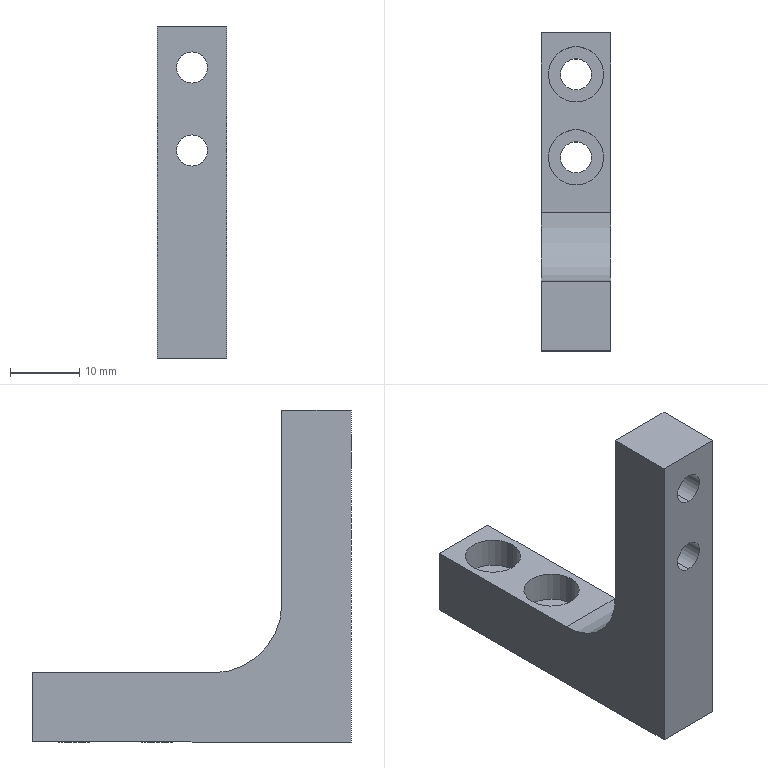Part | SolidWorks | features HoleWzd 2, Extrusion 1, Fillet 1, ICE 1 | 1 solid | 29 faces | box 10 x 46 x 48 mm | volume 7374 mm3 | cylinder 17 | plane 12 | commonest cylinder face diameters 4.5 x8 8 x8 20 x1
STEP:
#1=CARTESIAN_POINT('',(-4.,17.,-18.4));
#2=VERTEX_POINT('',#1);
#3=CARTESIAN_POINT('',(4.,17.,-18.4));
#4=VERTEX_POINT('',#3);
#5=CARTESIAN_POINT('',(0.,17.,-18.4));
#6=DIRECTION('',(0.,0.,1.));
#7=DIRECTION('',(1.,0.,0.));
#8=AXIS2_PLACEMENT_3D('',#5,#6,#7);
#9=CIRCLE('',#8,4.);
#10=EDGE_CURVE('',#2,#4,#9,.T.);
#11=ORIENTED_EDGE('',*,*,#10,.F.);
#12=CARTESIAN_POINT('',(-4.,17.,-14.));
#13=VERTEX_POINT('',#12);
#14=CARTESIAN_POINT('',(-4.,17.,-14.));
#15=DIRECTION('',(0.,0.,1.));
#16=VECTOR('',#15,1000.);
#17=LINE('',#14,#16);
#18=EDGE_CURVE('',#2,#13,#17,.T.);
#19=ORIENTED_EDGE('',*,*,#18,.T.);
#20=CARTESIAN_POINT('',(4.,17.,-14.));
#21=VERTEX_POINT('',#20);
#22=CARTESIAN_POINT('',(0.,17.,-14.));
#23=DIRECTION('',(0.,0.,1.));
#24=DIRECTION('',(1.,0.,0.));
#25=AXIS2_PLACEMENT_3D('',#22,#23,#24);
#26=CIRCLE('',#25,4.);
#27=EDGE_CURVE('',#13,#21,#26,.T.);
#28=ORIENTED_EDGE('',*,*,#27,.T.);
#29=CARTESIAN_POINT('',(4.,17.,-14.));
#30=DIRECTION('',(0.,0.,1.));
#31=VECTOR('',#30,1000.);
#32=LINE('',#29,#31);
#33=EDGE_CURVE('',#4,#21,#32,.T.);
#34=ORIENTED_EDGE('',*,*,#33,.F.);
#35=EDGE_LOOP('',(#11,#19,#28,#34));
#36=FACE_OUTER_BOUND('',#35,.T.);
#37=CARTESIAN_POINT('',(0.,17.,-14.));
#38=DIRECTION('',(0.,0.,1.));
#39=DIRECTION('',(1.,0.,0.));
#40=AXIS2_PLACEMENT_3D('',#37,#38,#39);
#41=CYLINDRICAL_SURFACE('',#40,4.);
#42=ADVANCED_FACE('',(#36),#41,.F.);
#43=CARTESIAN_POINT('',(-2.25,17.,-24.));
#44=VERTEX_POINT('',#43);
#45=CARTESIAN_POINT('',(2.25,17.,-24.));
#46=VERTEX_POINT('',#45);
#47=CARTESIAN_POINT('',(0.,17.,-24.));
#48=DIRECTION('',(0.,0.,1.));
#49=DIRECTION('',(1.,0.,0.));
#50=AXIS2_PLACEMENT_3D('',#47,#48,#49);
#51=CIRCLE('',#50,2.25);
#52=EDGE_CURVE('',#44,#46,#51,.T.);
#53=ORIENTED_EDGE('',*,*,#52,.F.);
#54=CARTESIAN_POINT('',(-2.25,17.,-18.4));
#55=VERTEX_POINT('',#54);
#56=CARTESIAN_POINT('',(-2.25,17.,-14.));
#57=DIRECTION('',(0.,0.,1.));
#58=VECTOR('',#57,1000.);
#59=LINE('',#56,#58);
#60=EDGE_CURVE('',#44,#55,#59,.T.);
#61=ORIENTED_EDGE('',*,*,#60,.T.);
#62=CARTESIAN_POINT('',(2.25,17.,-18.4));
#63=VERTEX_POINT('',#62);
#64=CARTESIAN_POINT('',(0.,17.,-18.4));
#65=DIRECTION('',(0.,0.,1.));
#66=DIRECTION('',(1.,0.,0.));
#67=AXIS2_PLACEMENT_3D('',#64,#65,#66);
#68=CIRCLE('',#67,2.25);
#69=EDGE_CURVE('',#55,#63,#68,.T.);
#70=ORIENTED_EDGE('',*,*,#69,.T.);
#71=CARTESIAN_POINT('',(2.25,17.,-14.));
#72=DIRECTION('',(0.,0.,1.));
#73=VECTOR('',#72,1000.);
#74=LINE('',#71,#73);
#75=EDGE_CURVE('',#46,#63,#74,.T.);
#76=ORIENTED_EDGE('',*,*,#75,.F.);
#77=EDGE_LOOP('',(#53,#61,#70,#76));
#78=FACE_OUTER_BOUND('',#77,.T.);
#79=CARTESIAN_POINT('',(0.,17.,-14.));
#80=DIRECTION('',(0.,0.,1.));
#81=DIRECTION('',(1.,0.,0.));
#82=AXIS2_PLACEMENT_3D('',#79,#80,#81);
#83=CYLINDRICAL_SURFACE('',#82,2.25);
#84=ADVANCED_FACE('',(#78),#83,.F.);
#85=CARTESIAN_POINT('',(-4.,5.,-18.4));
#86=VERTEX_POINT('',#85);
#87=CARTESIAN_POINT('',(4.,5.,-18.4));
#88=VERTEX_POINT('',#87);
#89=CARTESIAN_POINT('',(0.,5.,-18.4));
#90=DIRECTION('',(0.,0.,1.));
#91=DIRECTION('',(1.,0.,0.));
#92=AXIS2_PLACEMENT_3D('',#89,#90,#91);
#93=CIRCLE('',#92,4.);
#94=EDGE_CURVE('',#86,#88,#93,.T.);
#95=ORIENTED_EDGE('',*,*,#94,.F.);
#96=CARTESIAN_POINT('',(-4.,5.,-14.));
#97=VERTEX_POINT('',#96);
#98=CARTESIAN_POINT('',(-4.,5.,-14.));
#99=DIRECTION('',(0.,0.,1.));
#100=VECTOR('',#99,1000.);
#101=LINE('',#98,#100);
#102=EDGE_CURVE('',#86,#97,#101,.T.);
#103=ORIENTED_EDGE('',*,*,#102,.T.);
#104=CARTESIAN_POINT('',(4.,5.,-14.));
#105=VERTEX_POINT('',#104);
#106=CARTESIAN_POINT('',(0.,5.,-14.));
#107=DIRECTION('',(0.,0.,1.));
#108=DIRECTION('',(1.,0.,0.));
#109=AXIS2_PLACEMENT_3D('',#106,#107,#108);
#110=CIRCLE('',#109,4.);
#111=EDGE_CURVE('',#97,#105,#110,.T.);
#112=ORIENTED_EDGE('',*,*,#111,.T.);
#113=CARTESIAN_POINT('',(4.,5.,-14.));
#114=DIRECTION('',(0.,0.,1.));
#115=VECTOR('',#114,1000.);
#116=LINE('',#113,#115);
#117=EDGE_CURVE('',#88,#105,#116,.T.);
#118=ORIENTED_EDGE('',*,*,#117,.F.);
#119=EDGE_LOOP('',(#95,#103,#112,#118));
#120=FACE_OUTER_BOUND('',#119,.T.);
#121=CARTESIAN_POINT('',(0.,5.,-14.));
#122=DIRECTION('',(0.,0.,1.));
#123=DIRECTION('',(1.,0.,0.));
#124=AXIS2_PLACEMENT_3D('',#121,#122,#123);
#125=CYLINDRICAL_SURFACE('',#124,4.);
#126=ADVANCED_FACE('',(#120),#125,.F.);
#127=CARTESIAN_POINT('',(-2.25,5.,-24.));
#128=VERTEX_POINT('',#127);
#129=CARTESIAN_POINT('',(2.25,5.,-24.));
#130=VERTEX_POINT('',#129);
#131=CARTESIAN_POINT('',(0.,5.,-24.));
#132=DIRECTION('',(0.,0.,1.));
#133=DIRECTION('',(1.,0.,0.));
#134=AXIS2_PLACEMENT_3D('',#131,#132,#133);
#135=CIRCLE('',#134,2.25);
#136=EDGE_CURVE('',#128,#130,#135,.T.);
#137=ORIENTED_EDGE('',*,*,#136,.F.);
#138=CARTESIAN_POINT('',(-2.25,5.,-18.4));
#139=VERTEX_POINT('',#138);
#140=CARTESIAN_POINT('',(-2.25,5.,-14.));
#141=DIRECTION('',(0.,0.,1.));
#142=VECTOR('',#141,1000.);
#143=LINE('',#140,#142);
#144=EDGE_CURVE('',#128,#139,#143,.T.);
#145=ORIENTED_EDGE('',*,*,#144,.T.);
#146=CARTESIAN_POINT('',(2.25,5.,-18.4));
#147=VERTEX_POINT('',#146);
#148=CARTESIAN_POINT('',(0.,5.,-18.4));
#149=DIRECTION('',(0.,0.,1.));
#150=DIRECTION('',(1.,0.,0.));
#151=AXIS2_PLACEMENT_3D('',#148,#149,#150);
#152=CIRCLE('',#151,2.25);
#153=EDGE_CURVE('',#139,#147,#152,.T.);
#154=ORIENTED_EDGE('',*,*,#153,.T.);
#155=CARTESIAN_POINT('',(2.25,5.,-14.));
#156=DIRECTION('',(0.,0.,1.));
#157=VECTOR('',#156,1000.);
#158=LINE('',#155,#157);
#159=EDGE_CURVE('',#130,#147,#158,.T.);
#160=ORIENTED_EDGE('',*,*,#159,.F.);
#161=EDGE_LOOP('',(#137,#145,#154,#160));
#162=FACE_OUTER_BOUND('',#161,.T.);
#163=CARTESIAN_POINT('',(0.,5.,-14.));
#164=DIRECTION('',(0.,0.,1.));
#165=DIRECTION('',(1.,0.,0.));
#166=AXIS2_PLACEMENT_3D('',#163,#164,#165);
#167=CYLINDRICAL_SURFACE('',#166,2.25);
#168=ADVANCED_FACE('',(#162),#167,.F.);
#169=CARTESIAN_POINT('',(0.,-17.4,14.));
#170=VERTEX_POINT('',#169);
#171=CARTESIAN_POINT('',(0.,-17.4,22.));
#172=VERTEX_POINT('',#171);
#173=CARTESIAN_POINT('',(0.,-17.4,18.));
#174=DIRECTION('',(0.,1.,0.));
#175=DIRECTION('',(0.,0.,1.));
#176=AXIS2_PLACEMENT_3D('',#173,#174,#175);
#177=CIRCLE('',#176,4.);
#178=EDGE_CURVE('',#170,#172,#177,.T.);
#179=ORIENTED_EDGE('',*,*,#178,.F.);
#180=CARTESIAN_POINT('',(0.,-13.,14.));
#181=VERTEX_POINT('',#180);
#182=CARTESIAN_POINT('',(0.,-13.,14.));
#183=DIRECTION('',(0.,1.,0.));
#184=VECTOR('',#183,1000.);
#185=LINE('',#182,#184);
#186=EDGE_CURVE('',#170,#181,#185,.T.);
#187=ORIENTED_EDGE('',*,*,#186,.T.);
#188=CARTESIAN_POINT('',(0.,-13.,22.));
#189=VERTEX_POINT('',#188);
#190=CARTESIAN_POINT('',(0.,-13.,18.));
#191=DIRECTION('',(0.,1.,0.));
#192=DIRECTION('',(0.,0.,1.));
#193=AXIS2_PLACEMENT_3D('',#190,#191,#192);
#194=CIRCLE('',#193,4.);
#195=EDGE_CURVE('',#181,#189,#194,.T.);
#196=ORIENTED_EDGE('',*,*,#195,.T.);
#197=CARTESIAN_POINT('',(0.,-13.,22.));
#198=DIRECTION('',(0.,1.,0.));
#199=VECTOR('',#198,1000.);
#200=LINE('',#197,#199);
#201=EDGE_CURVE('',#172,#189,#200,.T.);
#202=ORIENTED_EDGE('',*,*,#201,.F.);
#203=EDGE_LOOP('',(#179,#187,#196,#202));
#204=FACE_OUTER_BOUND('',#203,.T.);
#205=CARTESIAN_POINT('',(0.,-13.,18.));
#206=DIRECTION('',(0.,1.,0.));
#207=DIRECTION('',(0.,0.,1.));
#208=AXIS2_PLACEMENT_3D('',#205,#206,#207);
#209=CYLINDRICAL_SURFACE('',#208,4.);
#210=ADVANCED_FACE('',(#204),#209,.F.);
#211=CARTESIAN_POINT('',(0.,-23.,15.75));
#212=VERTEX_POINT('',#211);
#213=CARTESIAN_POINT('',(0.,-23.,20.25));
#214=VERTEX_POINT('',#213);
#215=CARTESIAN_POINT('',(0.,-23.,18.));
#216=DIRECTION('',(0.,1.,0.));
#217=DIRECTION('',(0.,0.,1.));
#218=AXIS2_PLACEMENT_3D('',#215,#216,#217);
#219=CIRCLE('',#218,2.25);
#220=EDGE_CURVE('',#212,#214,#219,.T.);
#221=ORIENTED_EDGE('',*,*,#220,.F.);
#222=CARTESIAN_POINT('',(0.,-17.4,15.75));
#223=VERTEX_POINT('',#222);
#224=CARTESIAN_POINT('',(0.,-13.,15.75));
#225=DIRECTION('',(0.,1.,0.));
#226=VECTOR('',#225,1000.);
#227=LINE('',#224,#226);
#228=EDGE_CURVE('',#212,#223,#227,.T.);
#229=ORIENTED_EDGE('',*,*,#228,.T.);
#230=CARTESIAN_POINT('',(0.,-17.4,20.25));
#231=VERTEX_POINT('',#230);
#232=CARTESIAN_POINT('',(0.,-17.4,18.));
#233=DIRECTION('',(0.,1.,0.));
#234=DIRECTION('',(0.,0.,1.));
#235=AXIS2_PLACEMENT_3D('',#232,#233,#234);
#236=CIRCLE('',#235,2.25);
#237=EDGE_CURVE('',#223,#231,#236,.T.);
#238=ORIENTED_EDGE('',*,*,#237,.T.);
#239=CARTESIAN_POINT('',(0.,-13.,20.25));
#240=DIRECTION('',(0.,1.,0.));
#241=VECTOR('',#240,1000.);
#242=LINE('',#239,#241);
#243=EDGE_CURVE('',#214,#231,#242,.T.);
#244=ORIENTED_EDGE('',*,*,#243,.F.);
#245=EDGE_LOOP('',(#221,#229,#238,#244));
#246=FACE_OUTER_BOUND('',#245,.T.);
#247=CARTESIAN_POINT('',(0.,-13.,18.));
#248=DIRECTION('',(0.,1.,0.));
#249=DIRECTION('',(0.,0.,1.));
#250=AXIS2_PLACEMENT_3D('',#247,#248,#249);
#251=CYLINDRICAL_SURFACE('',#250,2.25);
#252=ADVANCED_FACE('',(#246),#251,.F.);
#253=CARTESIAN_POINT('',(0.,-17.4,2.));
#254=VERTEX_POINT('',#253);
#255=CARTESIAN_POINT('',(0.,-17.4,10.));
#256=VERTEX_POINT('',#255);
#257=CARTESIAN_POINT('',(0.,-17.4,6.));
#258=DIRECTION('',(0.,1.,0.));
#259=DIRECTION('',(0.,0.,1.));
#260=AXIS2_PLACEMENT_3D('',#257,#258,#259);
#261=CIRCLE('',#260,4.);
#262=EDGE_CURVE('',#254,#256,#261,.T.);
#263=ORIENTED_EDGE('',*,*,#262,.F.);
#264=CARTESIAN_POINT('',(0.,-13.,2.));
#265=VERTEX_POINT('',#264);
#266=CARTESIAN_POINT('',(0.,-13.,2.));
#267=DIRECTION('',(0.,1.,0.));
#268=VECTOR('',#267,1000.);
#269=LINE('',#266,#268);
#270=EDGE_CURVE('',#254,#265,#269,.T.);
#271=ORIENTED_EDGE('',*,*,#270,.T.);
#272=CARTESIAN_POINT('',(0.,-13.,10.));
#273=VERTEX_POINT('',#272);
#274=CARTESIAN_POINT('',(0.,-13.,6.));
#275=DIRECTION('',(0.,1.,0.));
#276=DIRECTION('',(0.,0.,1.));
#277=AXIS2_PLACEMENT_3D('',#274,#275,#276);
#278=CIRCLE('',#277,4.);
#279=EDGE_CURVE('',#265,#273,#278,.T.);
#280=ORIENTED_EDGE('',*,*,#279,.T.);
#281=CARTESIAN_POINT('',(0.,-13.,10.));
#282=DIRECTION('',(0.,1.,0.));
#283=VECTOR('',#282,1000.);
#284=LINE('',#281,#283);
#285=EDGE_CURVE('',#256,#273,#284,.T.);
#286=ORIENTED_EDGE('',*,*,#285,.F.);
#287=EDGE_LOOP('',(#263,#271,#280,#286));
#288=FACE_OUTER_BOUND('',#287,.T.);
#289=CARTESIAN_POINT('',(0.,-13.,6.));
#290=DIRECTION('',(0.,1.,0.));
#291=DIRECTION('',(0.,0.,1.));
#292=AXIS2_PLACEMENT_3D('',#289,#290,#291);
#293=CYLINDRICAL_SURFACE('',#292,4.);
#294=ADVANCED_FACE('',(#288),#293,.F.);
#295=CARTESIAN_POINT('',(0.,-23.,3.75));
#296=VERTEX_POINT('',#295);
#297=CARTESIAN_POINT('',(0.,-23.,8.25));
#298=VERTEX_POINT('',#297);
#299=CARTESIAN_POINT('',(0.,-23.,6.));
#300=DIRECTION('',(0.,1.,0.));
#301=DIRECTION('',(0.,0.,1.));
#302=AXIS2_PLACEMENT_3D('',#299,#300,#301);
#303=CIRCLE('',#302,2.25);
#304=EDGE_CURVE('',#296,#298,#303,.T.);
#305=ORIENTED_EDGE('',*,*,#304,.F.);
#306=CARTESIAN_POINT('',(0.,-17.4,3.75));
#307=VERTEX_POINT('',#306);
#308=CARTESIAN_POINT('',(0.,-13.,3.75));
#309=DIRECTION('',(0.,1.,0.));
#310=VECTOR('',#309,1000.);
#311=LINE('',#308,#310);
#312=EDGE_CURVE('',#296,#307,#311,.T.);
#313=ORIENTED_EDGE('',*,*,#312,.T.);
#314=CARTESIAN_POINT('',(0.,-17.4,8.25));
#315=VERTEX_POINT('',#314);
#316=CARTESIAN_POINT('',(0.,-17.4,6.));
#317=DIRECTION('',(0.,1.,0.));
#318=DIRECTION('',(0.,0.,1.));
#319=AXIS2_PLACEMENT_3D('',#316,#317,#318);
#320=CIRCLE('',#319,2.25);
#321=EDGE_CURVE('',#307,#315,#320,.T.);
#322=ORIENTED_EDGE('',*,*,#321,.T.);
#323=CARTESIAN_POINT('',(0.,-13.,8.25));
#324=DIRECTION('',(0.,1.,0.));
#325=VECTOR('',#324,1000.);
#326=LINE('',#323,#325);
#327=EDGE_CURVE('',#298,#315,#326,.T.);
#328=ORIENTED_EDGE('',*,*,#327,.F.);
#329=EDGE_LOOP('',(#305,#313,#322,#328));
#330=FACE_OUTER_BOUND('',#329,.T.);
#331=CARTESIAN_POINT('',(0.,-13.,6.));
#332=DIRECTION('',(0.,1.,0.));
#333=DIRECTION('',(0.,0.,1.));
#334=AXIS2_PLACEMENT_3D('',#331,#332,#333);
#335=CYLINDRICAL_SURFACE('',#334,2.25);
#336=ADVANCED_FACE('',(#330),#335,.F.);
#337=CARTESIAN_POINT('',(0.,17.,-24.));
#338=DIRECTION('',(0.,0.,1.));
#339=DIRECTION('',(1.,0.,0.));
#340=AXIS2_PLACEMENT_3D('',#337,#338,#339);
#341=CIRCLE('',#340,2.25);
#342=EDGE_CURVE('',#46,#44,#341,.T.);
#343=ORIENTED_EDGE('',*,*,#342,.T.);
#344=ORIENTED_EDGE('',*,*,#52,.T.);
#345=EDGE_LOOP('',(#343,#344));
#346=FACE_BOUND('',#345,.T.);
#347=CARTESIAN_POINT('',(0.,5.,-24.));
#348=DIRECTION('',(0.,0.,1.));
#349=DIRECTION('',(1.,0.,0.));
#350=AXIS2_PLACEMENT_3D('',#347,#348,#349);
#351=CIRCLE('',#350,2.25);
#352=EDGE_CURVE('',#130,#128,#351,.T.);
#353=ORIENTED_EDGE('',*,*,#352,.T.);
#354=ORIENTED_EDGE('',*,*,#136,.T.);
#355=EDGE_LOOP('',(#353,#354));
#356=FACE_BOUND('',#355,.T.);
#357=CARTESIAN_POINT('',(-5.,-23.,-24.));
#358=VERTEX_POINT('',#357);
#359=CARTESIAN_POINT('',(-5.,23.,-24.));
#360=VERTEX_POINT('',#359);
#361=CARTESIAN_POINT('',(-5.,23.,-24.));
#362=DIRECTION('',(0.,1.,0.));
#363=VECTOR('',#362,1000.);
#364=LINE('',#361,#363);
#365=EDGE_CURVE('',#358,#360,#364,.T.);
#366=ORIENTED_EDGE('',*,*,#365,.T.);
#367=CARTESIAN_POINT('',(5.,23.,-24.));
#368=VERTEX_POINT('',#367);
#369=CARTESIAN_POINT('',(5.,23.,-24.));
#370=DIRECTION('',(-1.,0.,0.));
#371=VECTOR('',#370,1000.);
#372=LINE('',#369,#371);
#373=EDGE_CURVE('',#368,#360,#372,.T.);
#374=ORIENTED_EDGE('',*,*,#373,.F.);
#375=CARTESIAN_POINT('',(5.,-23.,-24.));
#376=VERTEX_POINT('',#375);
#377=CARTESIAN_POINT('',(5.,23.,-24.));
#378=DIRECTION('',(0.,1.,0.));
#379=VECTOR('',#378,1000.);
#380=LINE('',#377,#379);
#381=EDGE_CURVE('',#376,#368,#380,.T.);
#382=ORIENTED_EDGE('',*,*,#381,.F.);
#383=CARTESIAN_POINT('',(5.,-23.,-24.));
#384=DIRECTION('',(-1.,0.,0.));
#385=VECTOR('',#384,1000.);
#386=LINE('',#383,#385);
#387=EDGE_CURVE('',#376,#358,#386,.T.);
#388=ORIENTED_EDGE('',*,*,#387,.T.);
#389=EDGE_LOOP('',(#366,#374,#382,#388));
#390=FACE_OUTER_BOUND('',#389,.T.);
#391=CARTESIAN_POINT('',(5.,23.,-24.));
#392=DIRECTION('',(0.,0.,1.));
#393=DIRECTION('',(0.,-1.,0.));
#394=AXIS2_PLACEMENT_3D('',#391,#392,#393);
#395=PLANE('',#394);
#396=ADVANCED_FACE('',(#346,#356,#390),#395,.F.);
#397=CARTESIAN_POINT('',(-5.,23.,-14.));
#398=VERTEX_POINT('',#397);
#399=CARTESIAN_POINT('',(-5.,23.,24.));
#400=DIRECTION('',(0.,0.,1.));
#401=VECTOR('',#400,1000.);
#402=LINE('',#399,#401);
#403=EDGE_CURVE('',#360,#398,#402,.T.);
#404=ORIENTED_EDGE('',*,*,#403,.T.);
#405=CARTESIAN_POINT('',(5.,23.,-14.));
#406=VERTEX_POINT('',#405);
#407=CARTESIAN_POINT('',(-5.,23.,-14.));
#408=DIRECTION('',(1.,0.,0.));
#409=VECTOR('',#408,1000.);
#410=LINE('',#407,#409);
#411=EDGE_CURVE('',#398,#406,#410,.T.);
#412=ORIENTED_EDGE('',*,*,#411,.T.);
#413=CARTESIAN_POINT('',(5.,23.,24.));
#414=DIRECTION('',(0.,0.,1.));
#415=VECTOR('',#414,1000.);
#416=LINE('',#413,#415);
#417=EDGE_CURVE('',#368,#406,#416,.T.);
#418=ORIENTED_EDGE('',*,*,#417,.F.);
#419=ORIENTED_EDGE('',*,*,#373,.T.);
#420=EDGE_LOOP('',(#404,#412,#418,#419));
#421=FACE_OUTER_BOUND('',#420,.T.);
#422=CARTESIAN_POINT('',(5.,23.,24.));
#423=DIRECTION('',(0.,-1.,0.));
#424=DIRECTION('',(0.,0.,-1.));
#425=AXIS2_PLACEMENT_3D('',#422,#423,#424);
#426=PLANE('',#425);
#427=ADVANCED_FACE('',(#421),#426,.F.);
#428=CARTESIAN_POINT('',(5.,-13.,24.));
#429=VERTEX_POINT('',#428);
#430=CARTESIAN_POINT('',(5.,-23.,24.));
#431=VERTEX_POINT('',#430);
#432=CARTESIAN_POINT('',(5.,23.,24.));
#433=DIRECTION('',(0.,-1.,0.));
#434=VECTOR('',#433,1000.);
#435=LINE('',#432,#434);
#436=EDGE_CURVE('',#429,#431,#435,.T.);
#437=ORIENTED_EDGE('',*,*,#436,.F.);
#438=CARTESIAN_POINT('',(-5.,-13.,24.));
#439=VERTEX_POINT('',#438);
#440=CARTESIAN_POINT('',(-5.,-13.,24.));
#441=DIRECTION('',(1.,0.,0.));
#442=VECTOR('',#441,1000.);
#443=LINE('',#440,#442);
#444=EDGE_CURVE('',#439,#429,#443,.T.);
#445=ORIENTED_EDGE('',*,*,#444,.F.);
#446=CARTESIAN_POINT('',(-5.,-23.,24.));
#447=VERTEX_POINT('',#446);
#448=CARTESIAN_POINT('',(-5.,23.,24.));
#449=DIRECTION('',(0.,-1.,0.));
#450=VECTOR('',#449,1000.);
#451=LINE('',#448,#450);
#452=EDGE_CURVE('',#439,#447,#451,.T.);
#453=ORIENTED_EDGE('',*,*,#452,.T.);
#454=CARTESIAN_POINT('',(5.,-23.,24.));
#455=DIRECTION('',(-1.,0.,0.));
#456=VECTOR('',#455,1000.);
#457=LINE('',#454,#456);
#458=EDGE_CURVE('',#431,#447,#457,.T.);
#459=ORIENTED_EDGE('',*,*,#458,.F.);
#460=EDGE_LOOP('',(#437,#445,#453,#459));
#461=FACE_OUTER_BOUND('',#460,.T.);
#462=CARTESIAN_POINT('',(5.,23.,24.));
#463=DIRECTION('',(0.,0.,-1.));
#464=DIRECTION('',(0.,1.,0.));
#465=AXIS2_PLACEMENT_3D('',#462,#463,#464);
#466=PLANE('',#465);
#467=ADVANCED_FACE('',(#461),#466,.F.);
#468=CARTESIAN_POINT('',(0.,-23.,18.));
#469=DIRECTION('',(0.,1.,0.));
#470=DIRECTION('',(0.,0.,1.));
#471=AXIS2_PLACEMENT_3D('',#468,#469,#470);
#472=CIRCLE('',#471,2.25);
#473=EDGE_CURVE('',#214,#212,#472,.T.);
#474=ORIENTED_EDGE('',*,*,#473,.T.);
#475=ORIENTED_EDGE('',*,*,#220,.T.);
#476=EDGE_LOOP('',(#474,#475));
#477=FACE_BOUND('',#476,.T.);
#478=CARTESIAN_POINT('',(0.,-23.,6.));
#479=DIRECTION('',(0.,1.,0.));
#480=DIRECTION('',(0.,0.,1.));
#481=AXIS2_PLACEMENT_3D('',#478,#479,#480);
#482=CIRCLE('',#481,2.25);
#483=EDGE_CURVE('',#298,#296,#482,.T.);
#484=ORIENTED_EDGE('',*,*,#483,.T.);
#485=ORIENTED_EDGE('',*,*,#304,.T.);
#486=EDGE_LOOP('',(#484,#485));
#487=FACE_BOUND('',#486,.T.);
#488=CARTESIAN_POINT('',(-5.,-23.,24.));
#489=DIRECTION('',(0.,0.,-1.));
#490=VECTOR('',#489,1000.);
#491=LINE('',#488,#490);
#492=EDGE_CURVE('',#447,#358,#491,.T.);
#493=ORIENTED_EDGE('',*,*,#492,.T.);
#494=ORIENTED_EDGE('',*,*,#387,.F.);
#495=CARTESIAN_POINT('',(5.,-23.,24.));
#496=DIRECTION('',(0.,0.,-1.));
#497=VECTOR('',#496,1000.);
#498=LINE('',#495,#497);
#499=EDGE_CURVE('',#431,#376,#498,.T.);
#500=ORIENTED_EDGE('',*,*,#499,.F.);
#501=ORIENTED_EDGE('',*,*,#458,.T.);
#502=EDGE_LOOP('',(#493,#494,#500,#501));
#503=FACE_OUTER_BOUND('',#502,.T.);
#504=CARTESIAN_POINT('',(5.,-23.,24.));
#505=DIRECTION('',(0.,1.,0.));
#506=DIRECTION('',(0.,0.,1.));
#507=AXIS2_PLACEMENT_3D('',#504,#505,#506);
#508=PLANE('',#507);
#509=ADVANCED_FACE('',(#477,#487,#503),#508,.F.);
#510=CARTESIAN_POINT('',(5.,-3.,-14.));
#511=VERTEX_POINT('',#510);
#512=CARTESIAN_POINT('',(5.,23.,-14.));
#513=DIRECTION('',(0.,1.,0.));
#514=VECTOR('',#513,1000.);
#515=LINE('',#512,#514);
#516=EDGE_CURVE('',#511,#406,#515,.T.);
#517=ORIENTED_EDGE('',*,*,#516,.F.);
#518=CARTESIAN_POINT('',(5.,-13.,-4.));
#519=VERTEX_POINT('',#518);
#520=CARTESIAN_POINT('',(5.,-3.,-4.));
#521=DIRECTION('',(-1.,0.,0.));
#522=DIRECTION('',(0.,0.,-1.));
#523=AXIS2_PLACEMENT_3D('',#520,#521,#522);
#524=CIRCLE('',#523,10.);
#525=EDGE_CURVE('',#511,#519,#524,.T.);
#526=ORIENTED_EDGE('',*,*,#525,.T.);
#527=CARTESIAN_POINT('',(5.,-13.,24.));
#528=DIRECTION('',(0.,0.,-1.));
#529=VECTOR('',#528,1000.);
#530=LINE('',#527,#529);
#531=EDGE_CURVE('',#429,#519,#530,.T.);
#532=ORIENTED_EDGE('',*,*,#531,.F.);
#533=ORIENTED_EDGE('',*,*,#436,.T.);
#534=ORIENTED_EDGE('',*,*,#499,.T.);
#535=ORIENTED_EDGE('',*,*,#381,.T.);
#536=ORIENTED_EDGE('',*,*,#417,.T.);
#537=EDGE_LOOP('',(#517,#526,#532,#533,#534,#535,#536));
#538=FACE_OUTER_BOUND('',#537,.T.);
#539=CARTESIAN_POINT('',(5.,0.,0.));
#540=DIRECTION('',(1.,0.,0.));
#541=DIRECTION('',(0.,0.,-1.));
#542=AXIS2_PLACEMENT_3D('',#539,#540,#541);
#543=PLANE('',#542);
#544=ADVANCED_FACE('',(#538),#543,.T.);
#545=CARTESIAN_POINT('',(-5.,-13.,-4.));
#546=VERTEX_POINT('',#545);
#547=CARTESIAN_POINT('',(-5.,-13.,24.));
#548=DIRECTION('',(0.,0.,-1.));
#549=VECTOR('',#548,1000.);
#550=LINE('',#547,#549);
#551=EDGE_CURVE('',#439,#546,#550,.T.);
#552=ORIENTED_EDGE('',*,*,#551,.T.);
#553=CARTESIAN_POINT('',(-5.,-3.,-14.));
#554=VERTEX_POINT('',#553);
#555=CARTESIAN_POINT('',(-5.,-3.,-4.));
#556=DIRECTION('',(1.,0.,0.));
#557=DIRECTION('',(0.,0.,-1.));
#558=AXIS2_PLACEMENT_3D('',#555,#556,#557);
#559=CIRCLE('',#558,10.);
#560=EDGE_CURVE('',#546,#554,#559,.T.);
#561=ORIENTED_EDGE('',*,*,#560,.T.);
#562=CARTESIAN_POINT('',(-5.,23.,-14.));
#563=DIRECTION('',(0.,1.,0.));
#564=VECTOR('',#563,1000.);
#565=LINE('',#562,#564);
#566=EDGE_CURVE('',#554,#398,#565,.T.);
#567=ORIENTED_EDGE('',*,*,#566,.T.);
#568=ORIENTED_EDGE('',*,*,#403,.F.);
#569=ORIENTED_EDGE('',*,*,#365,.F.);
#570=ORIENTED_EDGE('',*,*,#492,.F.);
#571=ORIENTED_EDGE('',*,*,#452,.F.);
#572=EDGE_LOOP('',(#552,#561,#567,#568,#569,#570,#571));
#573=FACE_OUTER_BOUND('',#572,.T.);
#574=CARTESIAN_POINT('',(-5.,0.,0.));
#575=DIRECTION('',(1.,0.,0.));
#576=DIRECTION('',(0.,0.,-1.));
#577=AXIS2_PLACEMENT_3D('',#574,#575,#576);
#578=PLANE('',#577);
#579=ADVANCED_FACE('',(#573),#578,.F.);
#580=CARTESIAN_POINT('',(0.,17.,-14.));
#581=DIRECTION('',(0.,0.,1.));
#582=DIRECTION('',(1.,0.,0.));
#583=AXIS2_PLACEMENT_3D('',#580,#581,#582);
#584=CIRCLE('',#583,4.);
#585=EDGE_CURVE('',#21,#13,#584,.T.);
#586=ORIENTED_EDGE('',*,*,#585,.F.);
#587=ORIENTED_EDGE('',*,*,#27,.F.);
#588=EDGE_LOOP('',(#586,#587));
#589=FACE_BOUND('',#588,.T.);
#590=CARTESIAN_POINT('',(0.,5.,-14.));
#591=DIRECTION('',(0.,0.,1.));
#592=DIRECTION('',(1.,0.,0.));
#593=AXIS2_PLACEMENT_3D('',#590,#591,#592);
#594=CIRCLE('',#593,4.);
#595=EDGE_CURVE('',#105,#97,#594,.T.);
#596=ORIENTED_EDGE('',*,*,#595,.F.);
#597=ORIENTED_EDGE('',*,*,#111,.F.);
#598=EDGE_LOOP('',(#596,#597));
#599=FACE_BOUND('',#598,.T.);
#600=ORIENTED_EDGE('',*,*,#566,.F.);
#601=CARTESIAN_POINT('',(5.,-3.,-14.));
#602=DIRECTION('',(1.,0.,0.));
#603=VECTOR('',#602,1000.);
#604=LINE('',#601,#603);
#605=EDGE_CURVE('',#554,#511,#604,.T.);
#606=ORIENTED_EDGE('',*,*,#605,.T.);
#607=ORIENTED_EDGE('',*,*,#516,.T.);
#608=ORIENTED_EDGE('',*,*,#411,.F.);
#609=EDGE_LOOP('',(#600,#606,#607,#608));
#610=FACE_OUTER_BOUND('',#609,.T.);
#611=CARTESIAN_POINT('',(-5.,23.,-14.));
#612=DIRECTION('',(0.,0.,-1.));
#613=DIRECTION('',(0.,1.,0.));
#614=AXIS2_PLACEMENT_3D('',#611,#612,#613);
#615=PLANE('',#614);
#616=ADVANCED_FACE('',(#589,#599,#610),#615,.F.);
#617=CARTESIAN_POINT('',(0.,-13.,18.));
#618=DIRECTION('',(0.,1.,0.));
#619=DIRECTION('',(0.,0.,1.));
#620=AXIS2_PLACEMENT_3D('',#617,#618,#619);
#621=CIRCLE('',#620,4.);
#622=EDGE_CURVE('',#189,#181,#621,.T.);
#623=ORIENTED_EDGE('',*,*,#622,.F.);
#624=ORIENTED_EDGE('',*,*,#195,.F.);
#625=EDGE_LOOP('',(#623,#624));
#626=FACE_BOUND('',#625,.T.);
#627=CARTESIAN_POINT('',(0.,-13.,6.));
#628=DIRECTION('',(0.,1.,0.));
#629=DIRECTION('',(0.,0.,1.));
#630=AXIS2_PLACEMENT_3D('',#627,#628,#629);
#631=CIRCLE('',#630,4.);
#632=EDGE_CURVE('',#273,#265,#631,.T.);
#633=ORIENTED_EDGE('',*,*,#632,.F.);
#634=ORIENTED_EDGE('',*,*,#279,.F.);
#635=EDGE_LOOP('',(#633,#634));
#636=FACE_BOUND('',#635,.T.);
#637=ORIENTED_EDGE('',*,*,#531,.T.);
#638=CARTESIAN_POINT('',(-5.,-13.,-4.));
#639=DIRECTION('',(-1.,0.,0.));
#640=VECTOR('',#639,1000.);
#641=LINE('',#638,#640);
#642=EDGE_CURVE('',#519,#546,#641,.T.);
#643=ORIENTED_EDGE('',*,*,#642,.T.);
#644=ORIENTED_EDGE('',*,*,#551,.F.);
#645=ORIENTED_EDGE('',*,*,#444,.T.);
#646=EDGE_LOOP('',(#637,#643,#644,#645));
#647=FACE_OUTER_BOUND('',#646,.T.);
#648=CARTESIAN_POINT('',(-5.,-13.,24.));
#649=DIRECTION('',(0.,-1.,0.));
#650=DIRECTION('',(0.,0.,-1.));
#651=AXIS2_PLACEMENT_3D('',#648,#649,#650);
#652=PLANE('',#651);
#653=ADVANCED_FACE('',(#626,#636,#647),#652,.F.);
#654=ORIENTED_EDGE('',*,*,#560,.F.);
#655=ORIENTED_EDGE('',*,*,#642,.F.);
#656=ORIENTED_EDGE('',*,*,#525,.F.);
#657=ORIENTED_EDGE('',*,*,#605,.F.);
#658=EDGE_LOOP('',(#654,#655,#656,#657));
#659=FACE_OUTER_BOUND('',#658,.T.);
#660=CARTESIAN_POINT('',(-5.,-3.,-4.));
#661=DIRECTION('',(-1.,0.,0.));
#662=DIRECTION('',(0.,0.,1.));
#663=AXIS2_PLACEMENT_3D('',#660,#661,#662);
#664=CYLINDRICAL_SURFACE('',#663,10.);
#665=ADVANCED_FACE('',(#659),#664,.F.);
#666=ORIENTED_EDGE('',*,*,#312,.F.);
#667=ORIENTED_EDGE('',*,*,#483,.F.);
#668=ORIENTED_EDGE('',*,*,#327,.T.);
#669=CARTESIAN_POINT('',(0.,-17.4,6.));
#670=DIRECTION('',(0.,1.,0.));
#671=DIRECTION('',(0.,0.,1.));
#672=AXIS2_PLACEMENT_3D('',#669,#670,#671);
#673=CIRCLE('',#672,2.25);
#674=EDGE_CURVE('',#315,#307,#673,.T.);
#675=ORIENTED_EDGE('',*,*,#674,.T.);
#676=EDGE_LOOP('',(#666,#667,#668,#675));
#677=FACE_OUTER_BOUND('',#676,.T.);
#678=CARTESIAN_POINT('',(0.,-13.,6.));
#679=DIRECTION('',(0.,1.,0.));
#680=DIRECTION('',(0.,0.,1.));
#681=AXIS2_PLACEMENT_3D('',#678,#679,#680);
#682=CYLINDRICAL_SURFACE('',#681,2.25);
#683=ADVANCED_FACE('',(#677),#682,.F.);
#684=ORIENTED_EDGE('',*,*,#674,.F.);
#685=ORIENTED_EDGE('',*,*,#321,.F.);
#686=EDGE_LOOP('',(#684,#685));
#687=FACE_BOUND('',#686,.T.);
#688=CARTESIAN_POINT('',(0.,-17.4,6.));
#689=DIRECTION('',(0.,1.,0.));
#690=DIRECTION('',(0.,0.,1.));
#691=AXIS2_PLACEMENT_3D('',#688,#689,#690);
#692=CIRCLE('',#691,4.);
#693=EDGE_CURVE('',#256,#254,#692,.T.);
#694=ORIENTED_EDGE('',*,*,#693,.T.);
#695=ORIENTED_EDGE('',*,*,#262,.T.);
#696=EDGE_LOOP('',(#694,#695));
#697=FACE_OUTER_BOUND('',#696,.T.);
#698=CARTESIAN_POINT('',(2.25,-17.4,6.));
#699=DIRECTION('',(0.,-1.,0.));
#700=DIRECTION('',(0.,0.,-1.));
#701=AXIS2_PLACEMENT_3D('',#698,#699,#700);
#702=PLANE('',#701);
#703=ADVANCED_FACE('',(#687,#697),#702,.F.);
#704=ORIENTED_EDGE('',*,*,#270,.F.);
#705=ORIENTED_EDGE('',*,*,#693,.F.);
#706=ORIENTED_EDGE('',*,*,#285,.T.);
#707=ORIENTED_EDGE('',*,*,#632,.T.);
#708=EDGE_LOOP('',(#704,#705,#706,#707));
#709=FACE_OUTER_BOUND('',#708,.T.);
#710=CARTESIAN_POINT('',(0.,-13.,6.));
#711=DIRECTION('',(0.,1.,0.));
#712=DIRECTION('',(0.,0.,1.));
#713=AXIS2_PLACEMENT_3D('',#710,#711,#712);
#714=CYLINDRICAL_SURFACE('',#713,4.);
#715=ADVANCED_FACE('',(#709),#714,.F.);
#716=ORIENTED_EDGE('',*,*,#228,.F.);
#717=ORIENTED_EDGE('',*,*,#473,.F.);
#718=ORIENTED_EDGE('',*,*,#243,.T.);
#719=CARTESIAN_POINT('',(0.,-17.4,18.));
#720=DIRECTION('',(0.,1.,0.));
#721=DIRECTION('',(0.,0.,1.));
#722=AXIS2_PLACEMENT_3D('',#719,#720,#721);
#723=CIRCLE('',#722,2.25);
#724=EDGE_CURVE('',#231,#223,#723,.T.);
#725=ORIENTED_EDGE('',*,*,#724,.T.);
#726=EDGE_LOOP('',(#716,#717,#718,#725));
#727=FACE_OUTER_BOUND('',#726,.T.);
#728=CARTESIAN_POINT('',(0.,-13.,18.));
#729=DIRECTION('',(0.,1.,0.));
#730=DIRECTION('',(0.,0.,1.));
#731=AXIS2_PLACEMENT_3D('',#728,#729,#730);
#732=CYLINDRICAL_SURFACE('',#731,2.25);
#733=ADVANCED_FACE('',(#727),#732,.F.);
#734=ORIENTED_EDGE('',*,*,#724,.F.);
#735=ORIENTED_EDGE('',*,*,#237,.F.);
#736=EDGE_LOOP('',(#734,#735));
#737=FACE_BOUND('',#736,.T.);
#738=CARTESIAN_POINT('',(0.,-17.4,18.));
#739=DIRECTION('',(0.,1.,0.));
#740=DIRECTION('',(0.,0.,1.));
#741=AXIS2_PLACEMENT_3D('',#738,#739,#740);
#742=CIRCLE('',#741,4.);
#743=EDGE_CURVE('',#172,#170,#742,.T.);
#744=ORIENTED_EDGE('',*,*,#743,.T.);
#745=ORIENTED_EDGE('',*,*,#178,.T.);
#746=EDGE_LOOP('',(#744,#745));
#747=FACE_OUTER_BOUND('',#746,.T.);
#748=CARTESIAN_POINT('',(2.25,-17.4,18.));
#749=DIRECTION('',(0.,-1.,0.));
#750=DIRECTION('',(0.,0.,-1.));
#751=AXIS2_PLACEMENT_3D('',#748,#749,#750);
#752=PLANE('',#751);
#753=ADVANCED_FACE('',(#737,#747),#752,.F.);
#754=ORIENTED_EDGE('',*,*,#186,.F.);
#755=ORIENTED_EDGE('',*,*,#743,.F.);
#756=ORIENTED_EDGE('',*,*,#201,.T.);
#757=ORIENTED_EDGE('',*,*,#622,.T.);
#758=EDGE_LOOP('',(#754,#755,#756,#757));
#759=FACE_OUTER_BOUND('',#758,.T.);
#760=CARTESIAN_POINT('',(0.,-13.,18.));
#761=DIRECTION('',(0.,1.,0.));
#762=DIRECTION('',(0.,0.,1.));
#763=AXIS2_PLACEMENT_3D('',#760,#761,#762);
#764=CYLINDRICAL_SURFACE('',#763,4.);
#765=ADVANCED_FACE('',(#759),#764,.F.);
#766=ORIENTED_EDGE('',*,*,#144,.F.);
#767=ORIENTED_EDGE('',*,*,#352,.F.);
#768=ORIENTED_EDGE('',*,*,#159,.T.);
#769=CARTESIAN_POINT('',(0.,5.,-18.4));
#770=DIRECTION('',(0.,0.,1.));
#771=DIRECTION('',(1.,0.,0.));
#772=AXIS2_PLACEMENT_3D('',#769,#770,#771);
#773=CIRCLE('',#772,2.25);
#774=EDGE_CURVE('',#147,#139,#773,.T.);
#775=ORIENTED_EDGE('',*,*,#774,.T.);
#776=EDGE_LOOP('',(#766,#767,#768,#775));
#777=FACE_OUTER_BOUND('',#776,.T.);
#778=CARTESIAN_POINT('',(0.,5.,-14.));
#779=DIRECTION('',(0.,0.,1.));
#780=DIRECTION('',(1.,0.,0.));
#781=AXIS2_PLACEMENT_3D('',#778,#779,#780);
#782=CYLINDRICAL_SURFACE('',#781,2.25);
#783=ADVANCED_FACE('',(#777),#782,.F.);
#784=ORIENTED_EDGE('',*,*,#774,.F.);
#785=ORIENTED_EDGE('',*,*,#153,.F.);
#786=EDGE_LOOP('',(#784,#785));
#787=FACE_BOUND('',#786,.T.);
#788=CARTESIAN_POINT('',(0.,5.,-18.4));
#789=DIRECTION('',(0.,0.,1.));
#790=DIRECTION('',(1.,0.,0.));
#791=AXIS2_PLACEMENT_3D('',#788,#789,#790);
#792=CIRCLE('',#791,4.);
#793=EDGE_CURVE('',#88,#86,#792,.T.);
#794=ORIENTED_EDGE('',*,*,#793,.T.);
#795=ORIENTED_EDGE('',*,*,#94,.T.);
#796=EDGE_LOOP('',(#794,#795));
#797=FACE_OUTER_BOUND('',#796,.T.);
#798=CARTESIAN_POINT('',(2.25,5.,-18.4));
#799=DIRECTION('',(0.,0.,-1.));
#800=DIRECTION('',(-1.,0.,0.));
#801=AXIS2_PLACEMENT_3D('',#798,#799,#800);
#802=PLANE('',#801);
#803=ADVANCED_FACE('',(#787,#797),#802,.F.);
#804=ORIENTED_EDGE('',*,*,#102,.F.);
#805=ORIENTED_EDGE('',*,*,#793,.F.);
#806=ORIENTED_EDGE('',*,*,#117,.T.);
#807=ORIENTED_EDGE('',*,*,#595,.T.);
#808=EDGE_LOOP('',(#804,#805,#806,#807));
#809=FACE_OUTER_BOUND('',#808,.T.);
#810=CARTESIAN_POINT('',(0.,5.,-14.));
#811=DIRECTION('',(0.,0.,1.));
#812=DIRECTION('',(1.,0.,0.));
#813=AXIS2_PLACEMENT_3D('',#810,#811,#812);
#814=CYLINDRICAL_SURFACE('',#813,4.);
#815=ADVANCED_FACE('',(#809),#814,.F.);
#816=ORIENTED_EDGE('',*,*,#60,.F.);
#817=ORIENTED_EDGE('',*,*,#342,.F.);
#818=ORIENTED_EDGE('',*,*,#75,.T.);
#819=CARTESIAN_POINT('',(0.,17.,-18.4));
#820=DIRECTION('',(0.,0.,1.));
#821=DIRECTION('',(1.,0.,0.));
#822=AXIS2_PLACEMENT_3D('',#819,#820,#821);
#823=CIRCLE('',#822,2.25);
#824=EDGE_CURVE('',#63,#55,#823,.T.);
#825=ORIENTED_EDGE('',*,*,#824,.T.);
#826=EDGE_LOOP('',(#816,#817,#818,#825));
#827=FACE_OUTER_BOUND('',#826,.T.);
#828=CARTESIAN_POINT('',(0.,17.,-14.));
#829=DIRECTION('',(0.,0.,1.));
#830=DIRECTION('',(1.,0.,0.));
#831=AXIS2_PLACEMENT_3D('',#828,#829,#830);
#832=CYLINDRICAL_SURFACE('',#831,2.25);
#833=ADVANCED_FACE('',(#827),#832,.F.);
#834=ORIENTED_EDGE('',*,*,#824,.F.);
#835=ORIENTED_EDGE('',*,*,#69,.F.);
#836=EDGE_LOOP('',(#834,#835));
#837=FACE_BOUND('',#836,.T.);
#838=CARTESIAN_POINT('',(0.,17.,-18.4));
#839=DIRECTION('',(0.,0.,1.));
#840=DIRECTION('',(1.,0.,0.));
#841=AXIS2_PLACEMENT_3D('',#838,#839,#840);
#842=CIRCLE('',#841,4.);
#843=EDGE_CURVE('',#4,#2,#842,.T.);
#844=ORIENTED_EDGE('',*,*,#843,.T.);
#845=ORIENTED_EDGE('',*,*,#10,.T.);
#846=EDGE_LOOP('',(#844,#845));
#847=FACE_OUTER_BOUND('',#846,.T.);
#848=CARTESIAN_POINT('',(2.25,17.,-18.4));
#849=DIRECTION('',(0.,0.,-1.));
#850=DIRECTION('',(-1.,0.,0.));
#851=AXIS2_PLACEMENT_3D('',#848,#849,#850);
#852=PLANE('',#851);
#853=ADVANCED_FACE('',(#837,#847),#852,.F.);
#854=ORIENTED_EDGE('',*,*,#18,.F.);
#855=ORIENTED_EDGE('',*,*,#843,.F.);
#856=ORIENTED_EDGE('',*,*,#33,.T.);
#857=ORIENTED_EDGE('',*,*,#585,.T.);
#858=EDGE_LOOP('',(#854,#855,#856,#857));
#859=FACE_OUTER_BOUND('',#858,.T.);
#860=CARTESIAN_POINT('',(0.,17.,-14.));
#861=DIRECTION('',(0.,0.,1.));
#862=DIRECTION('',(1.,0.,0.));
#863=AXIS2_PLACEMENT_3D('',#860,#861,#862);
#864=CYLINDRICAL_SURFACE('',#863,4.);
#865=ADVANCED_FACE('',(#859),#864,.F.);
#866=CLOSED_SHELL('',(#42,#84,#126,#168,#210,#252,#294,#336,#396,#427,#467,#509,#544,#579,#616,#653,#665,#683,#703,#715,#733,#753,#765,#783,#803,#815,#833,#853,#865));
#867=MANIFOLD_SOLID_BREP('',#866);
#868=CARTESIAN_POINT('',(0.,0.,0.));
#869=DIRECTION('',(0.,0.,1.));
#870=DIRECTION('',(1.,0.,0.));
#871=AXIS2_PLACEMENT_3D('',#868,#869,#870);
#872=(LENGTH_UNIT()NAMED_UNIT(*)SI_UNIT(.MILLI.,.METRE.));
#873=UNCERTAINTY_MEASURE_WITH_UNIT(LENGTH_MEASURE(0.00001),#872,'','');
#874=(NAMED_UNIT(*)PLANE_ANGLE_UNIT()SI_UNIT($,.RADIAN.));
#875=(NAMED_UNIT(*)SI_UNIT($,.STERADIAN.)SOLID_ANGLE_UNIT());
#876=(GEOMETRIC_REPRESENTATION_CONTEXT(3)GLOBAL_UNCERTAINTY_ASSIGNED_CONTEXT((#873))GLOBAL_UNIT_ASSIGNED_CONTEXT((#872,#874,#875))REPRESENTATION_CONTEXT('',''));
#877=ADVANCED_BREP_SHAPE_REPRESENTATION('',(#867,#871),#876);